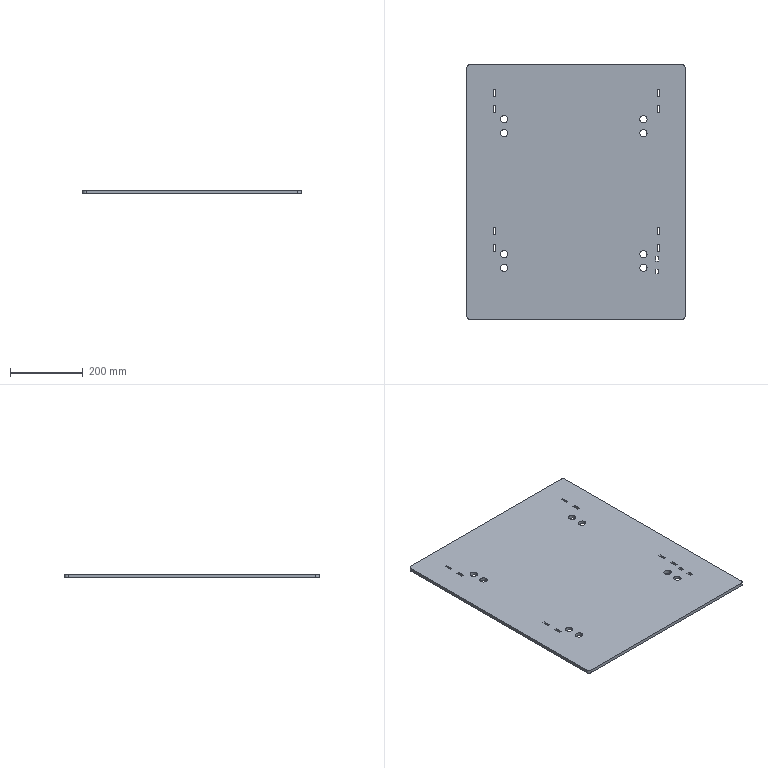Part | SolidWorks | features Cut 3, LPattern 2, Extrusion 1, Fillet 1 | 1 solid | 66 faces | box 600 x 700 x 9 mm | volume 3746150 mm3 | plane 46 | cylinder 20 | commonest cylinder face diameters 20 x20